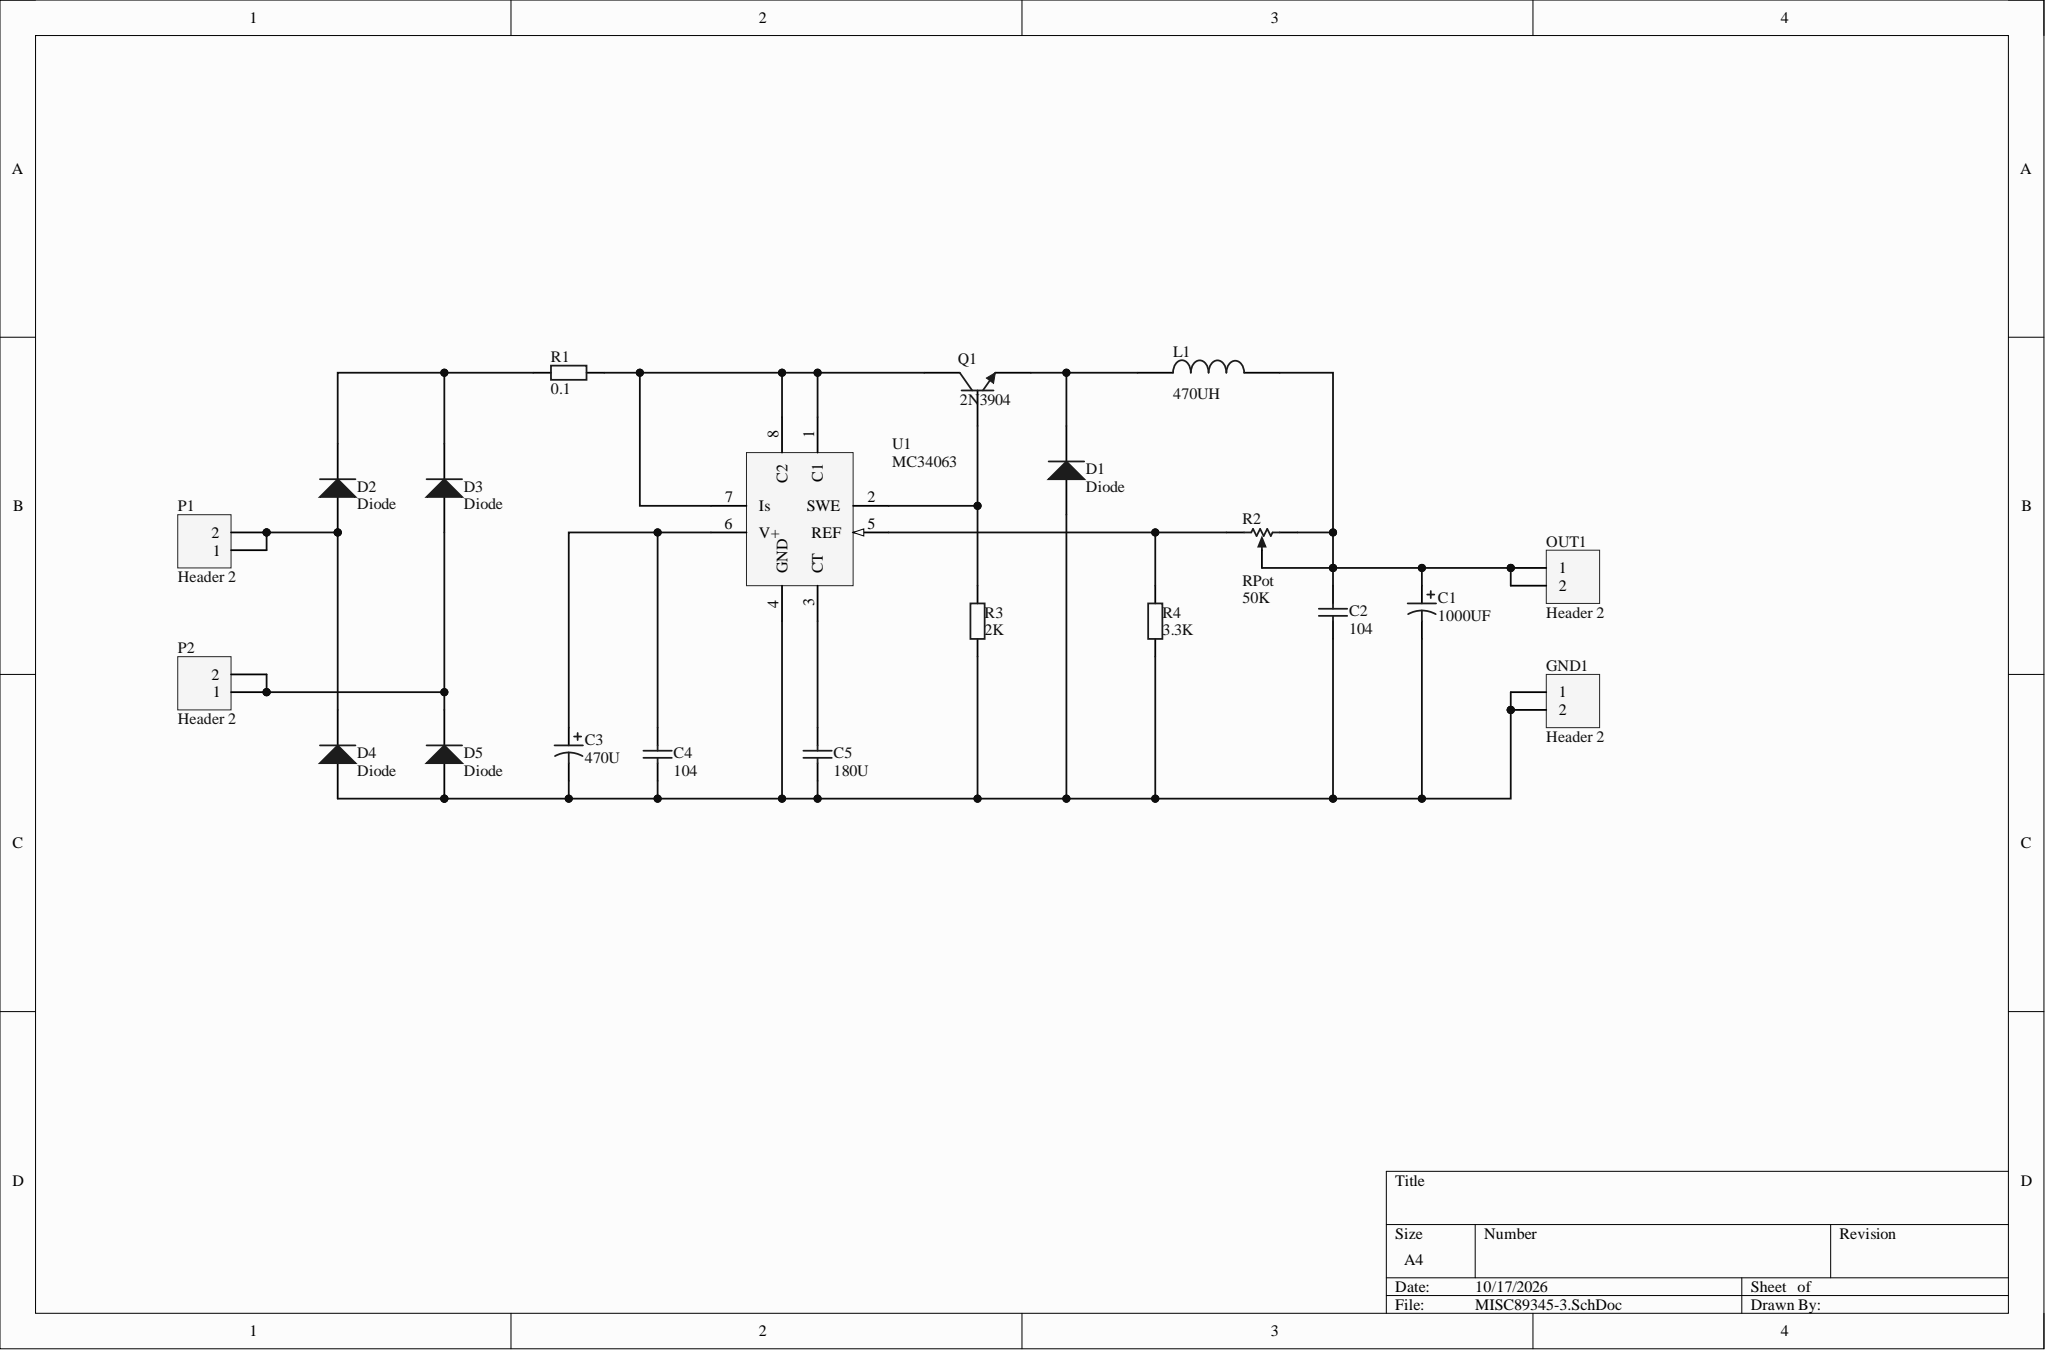Circuit board | Altium Designer | 21 parts | 11 nets
Bill of materials:
Comment,Description,Designator,Footprint,LibRef,Quantity
"1000UF","Polarized Capacitor (Surface Mount)","C1","C0805","Cap Pol3","1"
"104","Capacitor (Semiconductor SIM Model)","C2, C4","C1206","Cap Semi","2"
"470U","Polarized Capacitor (Surface Mount)","C3","C0805","Cap Pol3","1"
"180U","Capacitor (Semiconductor SIM Model)","C5","C1206","Cap Semi","1"
"Diode","Default Diode","D1, D2, D3, D4, D5","SMC","Diode","5"
"Header 2","Header, 2-Pin","GND1, OUT1, P1, P2","HDR1X2","Header 2","4"
"470UH","INDUCTOR","L1","AL0204","INDUCTOR","1"
"2N3904","NPN General Purpose Amplifier","Q1","TO-92A","2N3904","1"
"0.1","Resistor","R1","J1-0603","Res2","1"
"RPot","Potentiometer","R2","VR5","RPot","1"
"2K","Resistor","R3","J1-0603","Res2","1"
"3.3K","Resistor","R4","J1-0603","Res2","1"
"MC34063","DC-to-DC Converter Control Circuit","U1","693-02","MC34063U","1"
Netlist (Protel format):
[
C1
C0805
1000UF



]
[
C2
C1206
104



]
[
C3
C0805
470U



]
[
C4
C1206
104



]
[
C5
C1206
180U



]
[
D1
SMC
Diode



]
[
D2
SMC
Diode



]
[
D3
SMC
Diode



]
[
D4
SMC
Diode



]
[
D5
SMC
Diode



]
[
GND1
HDR1X2
Header 2



]
[
L1
AL0204
470UH



]
[
OUT1
HDR1X2
Header 2



]
[
P1
HDR1X2
Header 2



]
[
P2
HDR1X2
Header 2



]
[
Q1
TO-92A
2N3904



]
[
R1
J1-0603
0.1



]
[
R2
VR5
RPot



]
[
R3
J1-0603
2K



]
[
R4
J1-0603
3.3K



]
[
U1
693-02
MC34063



]
(
NetR2_1
R2-1
R4-1
U1-5
)
(
NetQ1_3
Q1-3
R1-1
U1-1
U1-7
U1-8
)
(
NetQ1_2
Q1-2
R3-2
U1-2
)
(
NetD3_1
D3-1
D5-2
P2-1
P2-2
)
(
NetD2_2
D2-2
D3-2
R1-2
)
(
NetD2_1
D2-1
D4-2
P1-1
P1-2
)
(
NetD1_2
D1-2
L1-1
Q1-1
)
(
NetC5_2
C5-2
U1-3
)
(
NetC3_1
C3-1
C4-2
U1-6
)
(
NetC1_2
C1-2
C2-1
C3-2
C4-1
C5-1
D1-1
D4-1
D5-1
GND1-1
GND1-2
R3-1
R4-2
U1-4
)
(
NetC1_1
C1-1
C2-2
L1-2
OUT1-1
OUT1-2
R2-2
R2-3
)